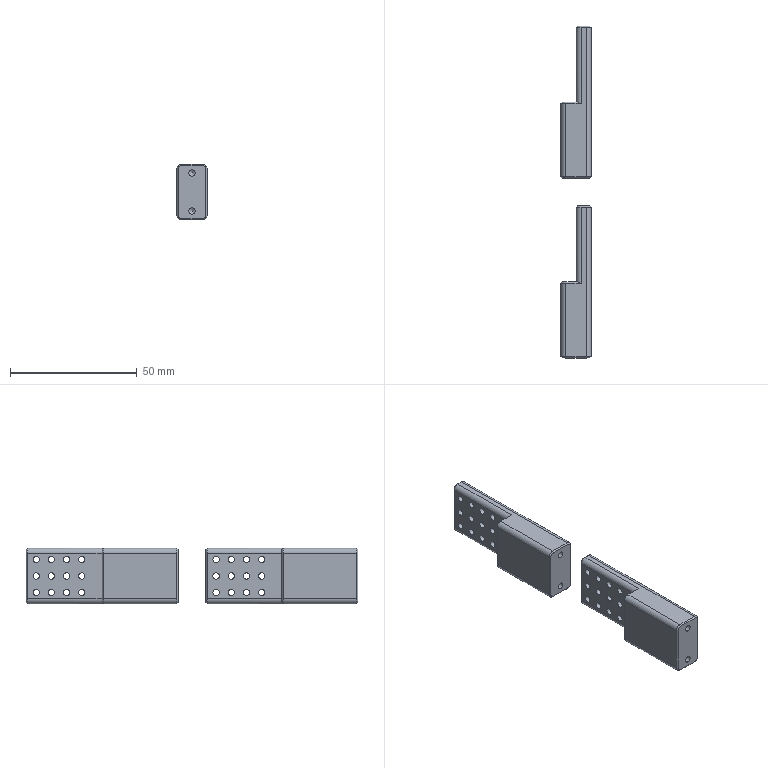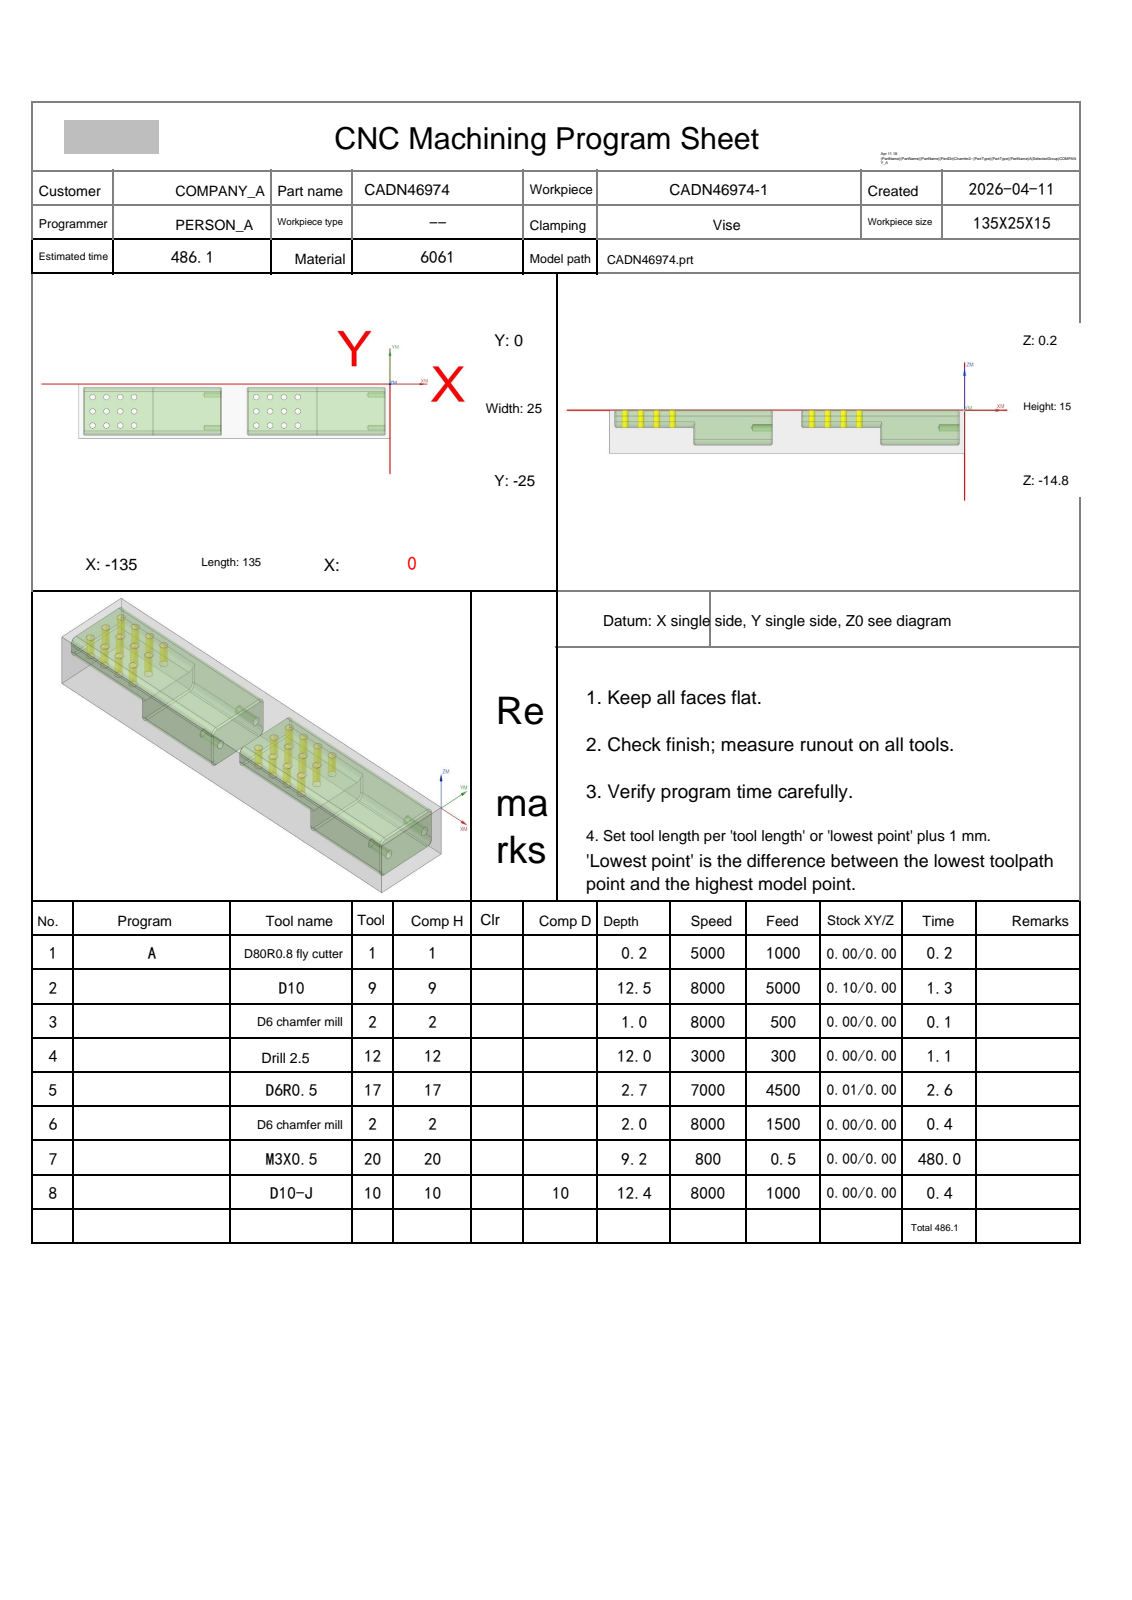NC program | NX | posted by the shop | part box 12 x 131 x 22 mm
Lines 673 to 2479 of 2479, first 1452 of 1807 lines:
N5 T17 M06
(D6R0.5  D=6. R=0.5 H=17 ce=0.01 di=0.00)
G00 G90 G54 X3.104 Y-17.401 M03 S7000
G43 H17 Z10.2
M08
Z.491
G01 Z-.009 F4500.
X3.1
G03 X.1 Y-20.397 I0.0 J-3.
G02 X.128 Y-20.959 I-5.567 J-.562
X.005 Y-22.127 I-5.596 J0.0
X-2.5 Y-24.221 I-2.59 J.553
G01 X-61.5
G02 X-64.069 Y-21.872 I.126 J2.717
G01 X-64.077 Y-21.814
X-64.091 Y-20.262
X-64.132 Z-.015
X-64.15 Z-.021
X-64.136 Y-21.732
G03 X-61.506 Y-24.336 I2.63 J.026
G01 X-2.5
G03 X.134 Y-21.627 I-.098 J2.73
G01 X.143 Y-20.397
X.193 Z-.038
X.185 Y-21.814
X.132 Y-22.159
G02 X-2.5 Y-24.443 I-2.718 J.473
G01 X-61.5
G02 X-64.184 Y-21.693 I.1 J2.782
G01 X-64.2 Y-20.262
X-64.224 Z-.048
X-64.242 Z-.058
X-64.227 Y-21.814
X-64.182 Y-22.159
G03 X-61.5 Y-24.546 I2.79 J.435
G01 X-2.5
G03 X.195 Y-22.071 I-.096 J2.81
G01 X.226 Y-21.814
X.24 Y-20.397
X.278 Z-.082
G02 X.304 Y-21.018 I-7.327 J-.621
X.184 Y-22.339 I-7.354 J0.0
X-2.5 Y-24.647 I-2.769 J.506
G01 X-61.5
G02 X-64.227 Y-22.159 I.094 J2.842
G01 X-64.269 Y-21.814
X-64.28 Y-20.298
X-64.317 Y-20.343 Z-.111
G03 X-64.341 Y-20.974 I8.456 J-.632
X-64.202 Y-22.504 I8.48 J0.0
X-61.5 Y-24.745 I2.81 J.639
G01 X-2.5
G03 X.219 Y-22.404 I-.075 J2.836
X.341 Y-21.019 I-7.816 J1.385
X.316 Y-20.397 I-7.937 J0.0
G01 X.342 Z-.127
X.359 Z-.143
X.349 Y-21.814
X.305 Y-22.159
G02 X-1.293 Y-24.55 I-3.063 J.317
X-2.5 Y-24.842 I-1.433 J3.287
G01 X-61.5
G02 X-64.034 Y-23.133 I.076 J2.846
G01 X-64.141 Y-22.84
G02 X-64.345 Y-21.713 I3.175 J1.158
G01 X-64.357 Y-20.394
X-64.395 Y-20.392 Z-.178
X-64.385 Y-21.656
G03 X-64.036 Y-23.254 I3.994 J.034
X-61.5 Y-24.937 I2.598 J1.163
G01 X-2.5
G03 X.065 Y-23.188 I-.07 J2.857
X.385 Y-21.633 I-3.774 J1.588
G01 X.395 Y-20.391
X.435 Z-.218
X.423 Y-21.814
X.384 Y-22.159
G02 X-.501 Y-24.157 I-3.438 J.329
X-2.478 Y-25.03 I-1.977 J1.801
G01 X-61.5
G02 X-63.948 Y-23.539 I.041 J2.822
X-64.387 Y-22.159 I3.309 J1.814
G01 X-64.422 Y-21.814
X-64.435 Y-20.394
X-64.478 Y-20.395 Z-.261
X-64.465 Y-21.814
G03 X-64.015 Y-23.539 I4.608 J.282
X-61.5 Y-25.122 I2.564 J1.285
G01 X-2.5
G03 X.009 Y-23.537 I-.042 J2.845
X.467 Y-21.615 I-3.965 J1.96
G01 X.478 Y-20.395
X.524 Y-20.397 Z-.307
X.513 Y-21.634
G02 X-.097 Y-23.837 I-4.424 J.04
X-2.499 Y-25.211 I-2.402 J1.412
G01 X-61.5
G02 X-64.066 Y-23.543 I.038 J2.866
X-64.514 Y-21.54 I4.451 J2.048
G01 X-64.524 Y-20.396
X-64.575 Y-20.398 Z-.357
G03 X-64.588 Y-20.988 I12.499 J-.59
X-64.562 Y-21.801 I12.513 J0.0
X-63.937 Y-23.884 I4.83 J.314
X-61.5 Y-25.298 I2.46 J1.433
G01 X-2.5
G03 X-.059 Y-23.884 I-.039 J2.882
X.567 Y-21.693 I-4.229 J2.392
X.582 Y-20.934 I-18.307 J.76
X.575 Y-20.398 I-18.323 J0.0
G01 X.628 Y-20.4 Z-.411
Y-21.469
G02 X-.004 Y-23.884 I-5.041 J.03
X-2.5 Y-25.383 I-2.519 J1.367
G01 X-61.5
G02 X-64.003 Y-23.879 I.031 J2.885
X-64.622 Y-21.633 I4.488 J2.447
X-64.636 Y-20.933 I17.84 J.7
X-64.628 Y-20.399 I17.853 J0.0
G01 X-64.685 Y-20.401 Z-.468
G03 X-64.693 Y-20.934 I17.258 J-.533
X-64.679 Y-21.641 I17.266 J0.0
X-63.845 Y-24.229 I5.08 J.208
X-61.5 Y-25.466 I2.373 J1.658
G01 X-2.5
G03 X-.063 Y-24.091 I-.032 J2.905
G01 X.054 Y-23.884
G03 X.667 Y-21.798 I-4.515 J2.46
X.698 Y-20.948 I-11.662 J.85
X.685 Y-20.401 I-11.693 J0.0
G01 X.745 Y-20.403 Z-.528
G02 X.758 Y-20.947 I-11.598 J-.544
X.694 Y-22.159 I-11.611 J0.0
X-.091 Y-24.229 I-5.507 J.906
X-2.5 Y-25.547 I-2.436 J1.593
G01 X-61.5
G02 X-63.901 Y-24.233 I.021 J2.89
X-64.729 Y-21.766 I4.355 J2.834
X-64.758 Y-20.947 I11.552 J.819
X-64.745 Y-20.399 I11.581 J0.0
G01 X-64.808 Y-20.406 Z-.591
G03 X-64.816 Y-20.874 I13.767 J-.467
X-64.756 Y-22.159 I13.775 J0.0
X-63.869 Y-24.368 I5.539 J.942
X-61.5 Y-25.625 I2.369 J1.604
G01 X-2.5
G03 X-.038 Y-24.229 I-.023 J2.91
X.757 Y-22.159 I-4.75 J3.012
X.821 Y-20.92 I-12.025 J1.239
X.808 Y-20.375 I-12.088 J0.0
G01 X.874 Y-20.415 Z-.658
G02 X.882 Y-20.873 I-13.64 J-.457
X.821 Y-22.159 I-13.648 J0.0
X.014 Y-24.229 I-5.474 J.943
G01 X-.22 Y-24.574
G02 X-2.5 Y-25.7 I-2.299 J1.786
G01 X-61.5
G02 X-63.687 Y-24.69 I.021 J2.917
X-64.82 Y-22.159 I4.359 J3.47
X-64.882 Y-20.878 I13.11 J1.282
X-64.874 Y-20.415 I13.173 J0.0
G01 X-64.909 Y-20.416 Z-.692
X-64.943 Y-20.417 Z-.727
G03 X-64.951 Y-20.882 I12.596 J-.464
X-64.886 Y-22.159 I12.605 J0.0
X-64.034 Y-24.288 I5.658 J1.031
G01 X-63.845 Y-24.574
G03 X-61.5 Y-25.772 I2.37 J1.744
G01 X-2.497
G03 X-.103 Y-24.488 I0.0 J2.872
G01 X.068 Y-24.229
G03 X.887 Y-22.159 I-4.524 J2.987
X.951 Y-20.876 I-12.929 J1.284
X.943 Y-20.417 I-12.992 J0.0
G01 X.979 Y-20.418 Z-.762
X1.013 Y-20.419 Z-.798
G02 X1.021 Y-20.863 I-12.618 J-.444
X.955 Y-22.159 I-12.626 J0.0
X.093 Y-24.276 I-5.299 J.922
X-2.5 Y-25.841 I-2.632 J1.43
G01 X-61.5
G02 X-63.9 Y-24.574 I.022 J2.948
G01 X-64.143 Y-24.196
G02 X-64.604 Y-23.345 I5.311 J3.423
X-65.011 Y-21.447 I4.296 J1.914
G01 X-65.013 Y-20.419
X-65.049 Y-20.42 Z-.833
X-65.084 Y-20.421 Z-.868
G03 X-65.092 Y-20.867 I11.906 J-.445
X-65.022 Y-22.159 I11.915 J0.0
X-64.034 Y-24.444 I5.388 J.974
X-61.5 Y-25.904 I2.56 J1.515
G01 X-2.5
G03 X-.323 Y-24.919 I-.013 J2.928
X.616 Y-23.44 I-5.066 J4.254
G01 X.662 Y-23.34
G03 X1.079 Y-21.464 I-4.106 J1.897
G01 X1.084 Y-20.422
X1.12 Y-20.423 Z-.904
X1.155 Y-20.424 Z-.939
G02 X1.162 Y-20.841 I-11.947 J-.417
X1.089 Y-22.159 I-11.954 J0.0
X-.001 Y-24.574 I-5.58 J1.065
X-2.5 Y-25.963 I-2.531 J1.611
G01 X-61.5
G02 X-64.034 Y-24.523 I.039 J3.017
X-65.09 Y-22.159 I4.492 J3.425
X-65.162 Y-20.837 I12.146 J1.322
X-65.155 Y-20.424 I12.217 J0.0
G01 X-65.191 Y-20.425 Z-.974
X-65.225 Y-20.426 Z-1.01
X-65.219 Y-21.469
G03 X-64.727 Y-23.47 I4.659 J.085
X-63.745 Y-24.966 I7.076 J3.575
X-61.503 Y-26.017 I2.242 J1.866
G01 X-2.5
G03 X-.215 Y-24.919 I-.02 J2.967
X.692 Y-23.539 I-6.554 J5.295
X1.219 Y-21.469 I-4.162 J2.162
G01 X1.226 Y-20.426
X1.261 Y-20.427 Z-1.045
X1.296 Y-20.428 Z-1.08
X1.289 Y-21.469
G02 X.753 Y-23.539 I-4.686 J.11
X-.262 Y-25.029 I-7.761 J4.197
X-2.497 Y-26.068 I-2.235 J1.884
G01 X-61.503
G02 X-63.757 Y-25.01 I0.0 J2.93
X-64.727 Y-23.588 I7.022 J5.833
X-65.288 Y-21.469 I4.103 J2.221
G01 X-65.296 Y-20.428
X-65.332 Y-20.429 Z-1.116
X-65.367 Y-20.43 Z-1.151
X-65.358 Y-21.469
G03 X-64.811 Y-23.539 I4.597 J.108
X-63.689 Y-25.132 I7.643 J4.191
X-61.504 Y-26.115 I2.185 J1.938
G01 X-2.5
G03 X-.253 Y-25.075 I-.024 J3.
G01 X-.128 Y-24.919
G03 X.787 Y-23.58 I-6.706 J5.558
X1.359 Y-21.469 I-4.009 J2.221
G01 X1.367 Y-20.43
X1.403 Y-20.431 Z-1.186
X1.438 Y-20.432 Z-1.222
X1.43 Y-21.431
G02 X.787 Y-23.671 I-4.346 J.036
X.184 Y-24.574 I-5.083 J2.737
X-.384 Y-25.264 I-6.247 J4.571
X-2.5 Y-26.159 I-2.14 J2.114
G01 X-61.5
G02 X-63.616 Y-25.264 I.024 J3.007
X-64.727 Y-23.782 I7.741 J6.956
X-65.427 Y-21.469 I3.958 J2.461
G01 X-65.431 Y-21.124
X-65.438 Y-20.432
X-65.473 Y-20.433 Z-1.257
X-65.508 Y-20.434 Z-1.293
X-65.497 Y-21.469
G03 X-64.924 Y-23.539 I4.366 J.095
X-63.687 Y-25.231 I9.099 J5.354
X-61.954 Y-26.162 I2.199 J2.016
G01 X-61.5 Y-26.199
X-2.5
X-2.272 Y-26.183
G03 X-.25 Y-25.158 I-.208 J2.918
G01 X-.048 Y-24.919
G03 X.924 Y-23.539 I-7.001 J5.959
X1.5 Y-21.469 I-3.831 J2.181
G01 X1.509 Y-20.434
X1.543 Y-20.583 Z-1.328
X1.576 Y-20.731 Z-1.363
X1.571 Y-21.469
G02 X.98 Y-23.539 I-4.32 J.114
X-.253 Y-25.202 I-9.003 J5.387
G01 X-.305 Y-25.264
G02 X-1.986 Y-26.19 I-2.21 J2.022
G01 X-2.5 Y-26.237
X-61.5
X-61.954 Y-26.201
G02 X-63.687 Y-25.274 I.469 J2.96
X-64.831 Y-23.791 I9.891 J8.817
X-65.547 Y-21.761 I3.655 J2.429
X-65.58 Y-21.027 I8.039 J.734
X-65.575 Y-20.727 I8.072 J0.0
G01 X-65.591 Y-20.896 Z-1.381
X-65.607 Y-21.064 Z-1.399
X-65.623 Y-21.232 Z-1.416
X-65.637 Y-21.401 Z-1.434
G03 X-65.037 Y-23.539 I4.149 J.01
X-63.653 Y-25.341 I9.631 J5.964
X-61.5 Y-26.271 I2.153 J2.028
G01 X-2.5
G03 X-.435 Y-25.431 I-.013 J2.991
X1.036 Y-23.539 I-8.047 J7.774
X1.641 Y-21.422 I-3.577 J2.168
G01 X1.649 Y-21.575 Z-1.444
X1.646 Y-21.729 Z-1.455
X1.639 Y-21.883 Z-1.465
X1.63 Y-22.037 Z-1.476
X1.615 Y-22.189 Z-1.486
X1.591 Y-22.339 Z-1.496
X1.559 Y-22.486 Z-1.507
G02 X.872 Y-23.884 I-4.54 J1.364
G01 X.44 Y-24.472
X.36 Y-24.574
X-.253 Y-25.281
G02 X-2.5 Y-26.304 I-2.264 J1.993
G01 X-61.503
G02 X-63.647 Y-25.381 I0.0 J2.95
X-64.874 Y-23.884 I9.924 J9.385
X-65.559 Y-22.49 I3.811 J2.74
G01 X-65.538 Y-22.628 Z-1.526
X-65.509 Y-22.765 Z-1.545
X-65.473 Y-22.898 Z-1.565
X-65.43 Y-23.028 Z-1.584
G03 X-64.927 Y-23.884 I4.787 J2.235
X-63.631 Y-25.43 I11.872 J8.636
X-61.502 Y-26.336 I2.13 J2.05
G01 X-2.5
G03 X-.401 Y-25.467 I-.006 J2.983
X.89 Y-23.93 I-10.286 J9.952
X1.431 Y-23.021 I-4.674 J3.398
G01 X1.402 Y-23.141 Z-1.611
X1.366 Y-23.257 Z-1.639
X1.317 Y-23.365 Z-1.666
G02 X.982 Y-23.884 I-3.452 J1.856
X-.382 Y-25.486 I-15.155 J11.531
X-2.5 Y-26.367 I-2.132 J2.139
G01 X-61.501
G02 X-63.631 Y-25.466 I0.0 J2.969
X-64.981 Y-23.884 I11.741 J11.393
X-65.32 Y-23.366 I3.833 J2.875
G01 X-65.281 Y-23.494 Z-1.709
X-65.228 Y-23.614 Z-1.752
G03 X-64.768 Y-24.229 I6.406 J4.313
G01 X-64.744 Y-24.252
G03 X-63.609 Y-25.518 I13.127 J10.626
X-61.503 Y-26.395 I2.106 J2.088
G01 X-2.5
G03 X-.593 Y-25.706 I-.016 J3.027
X-.392 Y-25.519 I-1.452 J1.765
G01 X-.149 Y-25.264
G03 X1.228 Y-23.618 I-10.789 J10.416
G01 X1.193 Y-23.718 Z-1.796
X1.148 Y-23.811 Z-1.84
G02 X-.253 Y-25.402 I-15.669 J12.394
G01 X-.289 Y-25.441
G02 X-2.495 Y-26.421 I-2.206 J1.993
G01 X-61.501
G02 X-63.626 Y-25.53 I0.0 J2.98
X-65.074 Y-23.911 I16.403 J16.117
G01 X-65.151 Y-23.805
X-65.12 Y-23.891 Z-1.886
X-65.081 Y-23.969 Z-1.931
G03 X-63.645 Y-25.538 I27.351 J23.594
X-61.502 Y-26.444 I2.144 J2.081
G01 X-2.496
G03 X-.28 Y-25.459 I0.0 J2.984
G01 X-.253 Y-25.429
G03 X1.098 Y-23.944 I-19.21 J18.822
G01 X1.058 Y-24.044 Z-2.026
G02 X-.332 Y-25.538 I-29.21 J25.791
X-2.5 Y-26.465 I-2.171 J2.08
G01 X-61.5
G02 X-63.687 Y-25.518 I.005 J3.012
X-65.043 Y-24.066 I34.442 J33.526
G01 X-65.005 Y-24.154 Z-2.122
G03 X-63.616 Y-25.609 I50.137 J46.44
X-61.5 Y-26.481 I2.122 J2.146
G01 X-2.5
G03 X-.383 Y-25.609 I-.006 J3.019
X1.012 Y-24.141 I-43.047 J42.298
G01 X.963 Y-24.23 Z-2.217
G03 X.44 Y-24.774 I18.578 J-18.365
G01 X.305 Y-24.919
G02 X-.446 Y-25.678 I-34.783 J33.665
X-2.5 Y-26.494 I-2.057 J2.184
G01 X-61.5
G02 X-63.629 Y-25.609 I.013 J3.035
X-64.963 Y-24.232 I99.236 J97.412
G01 X-64.939 Y-24.279 Z-2.311
X-64.858 Y-24.364
X-63.636 Y-25.609
G03 X-61.5 Y-26.503 I2.157 J2.156
G01 X-2.5
G03 X-.36 Y-25.609 I-.018 J3.051
G01 X-.315 Y-25.556
X-.253 Y-25.494
X.938 Y-24.278
X.926 Y-24.307 Z-2.406
X-.362 Y-25.614
G02 X-2.5 Y-26.508 I-2.138 J2.108
G01 X-61.506
G02 X-63.632 Y-25.619 I0.0 J2.987
G01 X-64.925 Y-24.309
X-64.915 Y-24.335 Z-2.5
X-64.677 Y-24.574
X-63.586 Y-25.67
G03 X-61.5 Y-26.51 I2.088 J2.174
G01 X-2.5
G03 X-.423 Y-25.678 I0.0 J3.007
G01 X.915 Y-24.333
G00 Z10.2
X-67.104 Y-7.564
Z.491
G01 Z-.009
X-67.094
G03 X-64.094 Y-4.601 I0.0 J3.
G01 X-64.077 Y-3.186
X-64.063 Y-3.091
G02 X-61.5 Y-.779 I2.687 J-.403
G01 X-2.5
G02 X.081 Y-3.186 I-.124 J-2.72
G01 X.093 Y-3.316
X.101 Y-4.6
X.148 Z-.021
X.134 Y-3.365
G03 X-2.5 Y-.664 I-2.733 J-.031
G01 X-61.507
G03 X-64.136 Y-3.268 I0.0 J-2.629
G01 X-64.149 Y-4.599
X-64.199 Z-.038
X-64.182 Y-3.186
X-64.149 Y-2.943
G02 X-61.5 Y-.557 I2.739 J-.377
G01 X-2.5
G02 X.132 Y-2.841 I-.085 J-2.757
G01 X.185 Y-3.186
X.197 Y-4.6
X.241 Z-.058
X.226 Y-3.186
X.195 Y-2.929
G03 X-2.5 Y-.454 I-2.791 J-.335
G01 X-61.5
G03 X-64.182 Y-2.841 I.108 J-2.822
G01 X-64.227 Y-3.186
X-64.24 Y-4.599
X-64.266 Y-4.6 Z-.07
X-64.282 Y-4.601 Z-.082
X-64.269 Y-3.186
X-64.227 Y-2.841
G02 X-61.5 Y-.353 I2.821 J-.354
G01 X-2.5
G02 X.226 Y-2.841 I-.105 J-2.853
G01 X.272 Y-3.186
X.283 Y-4.6
X.32 Z-.111
X.312 Y-3.186
X.272 Y-2.841
G03 X-2.5 Y-.255 I-2.874 J-.302
G01 X-61.5
G03 X-64.202 Y-2.496 I.108 J-2.88
X-64.34 Y-4.003 I8.134 J-1.507
X-64.319 Y-4.601 I8.272 J0.0
G01 X-64.342 Y-4.6 Z-.127
X-64.357 Y-4.599 Z-.143
X-64.344 Y-3.186
X-64.31 Y-2.841
G02 X-62.647 Y-.418 I3.103 J-.348
X-61.5 Y-.158 I1.423 J-3.623
G01 X-2.5
G02 X-.003 Y-1.801 I-.058 J-2.807
X.351 Y-3.404 I-3.58 J-1.63
G01 X.359 Y-4.6
X.395 Y-4.631 Z-.178
G03 X.414 Y-4.04 I-9.48 J.591
X.287 Y-2.496 I-9.498 J0.0
X-2.5 Y-.063 I-2.904 J-.515
G01 X-61.5
G03 X-63.324 Y-.771 I.083 J-2.92
X-64.347 Y-2.841 I2.273 J-2.41
G01 X-64.383 Y-3.186
X-64.395 Y-4.608
X-64.435 Y-4.606 Z-.218
X-64.422 Y-3.186
X-64.387 Y-2.841
G02 X-63.493 Y-.84 I3.472 J-.351
X-61.522 Y.03 I1.971 J-1.798
G01 X-2.5
G02 X.095 Y-1.75 I-.057 J-2.864
X.424 Y-3.392 I-4.11 J-1.68
G01 X.435 Y-4.604
X.478 Y-4.606 Z-.261
X.467 Y-3.385
G03 X.009 Y-1.463 I-4.423 J-.038
X-2.5 Y.122 I-2.551 J-1.261
G01 X-61.5
G03 X-64.015 Y-1.461 I.049 J-2.868
X-64.465 Y-3.186 I4.158 J-2.007
G01 X-64.478 Y-4.605
X-64.501 Y-4.604 Z-.284
X-64.524 Z-.307
X-64.514 Y-3.46
G02 X-64.066 Y-1.457 I4.9 J-.045
X-61.5 Y.211 I2.604 J-1.198
G01 X-2.5
G02 X-.085 Y-1.184 I0.0 J-2.788
X.512 Y-3.186 I-3.911 J-2.256
G01 X.524 Y-4.605
X.575 Y-4.603 Z-.357
G03 X.582 Y-4.069 I-18.545 J.534
X.567 Y-3.309 I-18.553 J0.0
X-.059 Y-1.116 I-4.854 J-.199
X-2.5 Y.298 I-2.48 J-1.468
G01 X-61.5
G03 X-63.937 Y-1.116 I.024 J-2.847
X-64.561 Y-3.186 I4.205 J-2.398
X-64.582 Y-4.067 I18.267 J-.881
X-64.575 Y-4.602 I18.288 J0.0
G01 X-64.601 Z-.384
X-64.628 Y-4.601 Z-.411
G02 X-64.636 Y-4.066 I17.668 J.535
X-64.622 Y-3.365 I17.676 J0.0
X-64.003 Y-1.121 I5.109 J-.203
X-61.5 Y.383 I2.534 J-1.381
G01 X-2.5
G02 X-.004 Y-1.116 I-.023 J-2.866
X.628 Y-3.531 I-4.409 J-2.445
G01 Y-4.602
X.685 Y-4.6 Z-.468
G03 X.698 Y-4.05 I-11.6 J.55
X.667 Y-3.195 I-11.613 J0.0
X.021 Y-1.058 I-5.111 J-.377
G01 X-.063 Y-.909
G03 X-2.5 Y.466 I-2.47 J-1.53
G01 X-61.5
G03 X-63.845 Y-.771 I.028 J-2.895
X-64.679 Y-3.357 I4.247 J-2.797
X-64.693 Y-4.065 I17.096 J-.708
X-64.685 Y-4.599 I17.111 J0.0
G01 X-64.745 Y-4.601 Z-.528
G02 X-64.758 Y-4.058 I11.732 J.544
X-64.729 Y-3.236 I11.745 J0.0
X-63.901 Y-.767 I5.18 J-.363
X-61.5 Y.547 I2.422 J-1.577
G01 X-2.5
G02 X-.091 Y-.771 I-.027 J-2.911
X.694 Y-2.841 I-4.722 J-2.976
X.758 Y-4.05 I-11.438 J-1.21
X.745 Y-4.598 I-11.502 J0.0
G01 X.808 Y-4.626 Z-.591
G03 X.821 Y-4.071 I-11.761 J.555
X.757 Y-2.841 I-11.774 J0.0
X-.038 Y-.771 I-5.545 J-.942
X-2.5 Y.625 I-2.485 J-1.515
G01 X-61.5
G03 X-63.869 Y-.632 I0.0 J-2.861
X-64.756 Y-2.841 I4.653 J-3.152
X-64.816 Y-4.128 I13.787 J-1.288
X-64.808 Y-4.594 I13.847 J0.0
G01 X-64.842 Y-4.589 Z-.624
X-64.874 Y-4.585 Z-.658
G02 X-64.882 Y-4.129 I13.336 J.456
X-64.82 Y-2.841 I13.343 J0.0
X-63.687 Y-.31 I5.493 J-.941
X-61.5 Y.7 I2.208 J-1.907
G01 X-2.5
G02 X-.22 Y-.426 I-.019 J-2.911
G01 X-.049 Y-.678
G02 X.821 Y-2.841 I-4.572 J-3.096
X.882 Y-4.124 I-13.479 J-1.283
X.874 Y-4.586 I-13.54 J0.0
G01 X.909 Y-4.585 Z-.692
X.942 Y-4.584 Z-.727
X.943 Y-3.876
X.941 Y-3.531
G03 X.093 Y-.81 I-5.137 J-.108
G01 X.068 Y-.771
G03 X-2.5 Y.772 I-2.6 J-1.419
G01 X-61.507
G03 X-63.909 Y-.522 I0.0 J-2.876
G01 X-64.034 Y-.712
G03 X-64.886 Y-2.841 I4.809 J-3.162
X-64.951 Y-4.128 I12.765 J-1.287
X-64.943 Y-4.583 I12.83 J0.0
G01 X-64.979 Y-4.582 Z-.762
X-65.014 Y-4.581 Z-.798
X-65.011 Y-3.531
G02 X-64.51 Y-1.461 I4.683 J-.038
X-64.034 Y-.634 I4.75 J-2.182
X-61.5 Y.841 I2.559 J-1.483
G01 X-2.5
G02 X.093 Y-.724 I-.038 J-2.995
X.954 Y-2.841 I-4.435 J-3.037
X1.021 Y-4.136 I-12.618 J-1.296
X1.013 Y-4.581 I-12.684 J0.0
G01 X1.049 Y-4.58 Z-.833
X1.084 Y-4.579 Z-.868
X1.079 Y-3.506
G03 X.723 Y-1.793 I-4.381 J-.017
X-.205 Y-.219 I-6.635 J-2.852
X-2.497 Y.904 I-2.292 J-1.778
G01 X-61.5
G03 X-64.034 Y-.556 I.026 J-2.974
X-65.022 Y-2.841 I4.405 J-3.262
X-65.092 Y-4.146 I12.137 J-1.305
X-65.085 Y-4.578 I12.207 J0.0
G01 X-65.121 Y-4.577 Z-.904
X-65.155 Y-4.576 Z-.939
G02 X-65.163 Y-4.155 I11.947 J.421
X-65.09 Y-2.841 I11.955 J0.0
X-64.034 Y-.477 I5.555 J-1.066
X-61.5 Y.963 I2.573 J-1.577
G01 X-2.5
G02 X-.001 Y-.426 I-.031 J-3.
X1.089 Y-2.841 I-4.49 J-3.479
X1.162 Y-4.145 I-11.551 J-1.304
X1.154 Y-4.577 I-11.624 J0.0
G01 X1.19 Y-4.575 Z-.974
X1.225 Y-4.574 Z-1.01
X1.218 Y-3.531
G03 X.692 Y-1.461 I-4.689 J-.091
X-.215 Y-.081 I-7.45 J-3.908
X-2.5 Y1.017 I-2.304 J-1.868
G01 X-61.503
G03 X-63.745 Y-.034 I0.0 J-2.917
X-64.727 Y-1.53 I6.094 J-5.072
X-65.22 Y-3.531 I4.172 J-2.089
G01 X-65.226 Y-4.574
X-65.262 Y-4.573 Z-1.045
X-65.297 Y-4.572 Z-1.08
X-65.29 Y-3.531
G02 X-64.727 Y-1.412 I4.676 J-.108
X-63.758 Y.008 I7.994 J-4.412
X-61.502 Y1.068 I2.256 J-1.873
G01 X-2.497
G02 X-.263 Y.029 I0.0 J-2.923
X.752 Y-1.461 I-6.732 J-5.678
X1.288 Y-3.531 I-4.143 J-2.176
G01 X1.296 Y-4.572
X1.331 Y-4.571 Z-1.116
X1.366 Y-4.57 Z-1.151
X1.358 Y-3.531
G03 X.787 Y-1.421 I-4.567 J-.104
X-.128 Y-.081 I-7.609 J-4.21
G01 X-.253 Y.075
G03 X-2.5 Y1.115 I-2.271 J-1.96
G01 X-61.503
G03 X-63.689 Y.132 I0.0 J-2.921
X-64.811 Y-1.461 I6.523 J-5.784
X-65.36 Y-3.531 I4.068 J-2.187
G01 X-65.368 Y-4.57
X-65.403 Y-4.569 Z-1.186
X-65.439 Y-4.568 Z-1.222
X-65.435 Y-3.876
X-65.43 Y-3.531
G02 X-64.727 Y-1.218 I4.68 J-.16
X-63.616 Y.264 I8.855 J-5.475
X-61.5 Y1.159 I2.141 J-2.114
G01 X-2.5
G02 X-.253 Y.12 I-.022 J-2.998
X.295 Y-.568 I-12.955 J-10.877
X1.029 Y-1.792 I-5.36 J-4.044
X1.427 Y-3.531 I-3.916 J-1.812
G01 X1.437 Y-4.567
X1.507 Y-4.532 Z-1.293
X1.497 Y-3.531
G03 X.923 Y-1.461 I-4.374 J-.097
X-.048 Y-.081 I-7.945 J-4.558
G01 X-.251 Y.159
G03 X-2.27 Y1.183 I-2.226 J-1.889
G01 X-2.5 Y1.199
X-61.5
X-61.954 Y1.162
G03 X-63.687 Y.231 I.468 J-2.951
X-64.924 Y-1.461 I7.866 J-7.049
X-65.501 Y-3.531 I3.83 J-2.182
G01 X-65.509 Y-4.566
X-65.544 Y-4.416 Z-1.328
X-65.577 Y-4.267 Z-1.363
X-65.572 Y-3.531
G02 X-64.981 Y-1.461 I4.303 J-.109
X-63.696 Y.264 I9.768 J-5.937
X-61.954 Y1.201 I2.209 J-2.02
G01 X-61.5 Y1.237
X-2.5
G02 X-1.324 Y.989 I-.05 J-3.154
X-.344 Y.301 I-1.103 J-2.616
X.899 Y-1.322 I-8.053 J-7.452
X1.546 Y-3.24 I-3.691 J-2.314
X1.58 Y-3.969 I-7.987 J-.729
X1.574 Y-4.263 I-8.021 J0.0
G01 X1.591 Y-4.098 Z-1.381
X1.606 Y-3.933 Z-1.399
X1.622 Y-3.768 Z-1.416
X1.637 Y-3.604 Z-1.434
G03 X1.036 Y-1.461 I-4.125 J-.001
X-.43 Y.427 I-9.571 J-5.917
X-2.5 Y1.271 I-2.083 J-2.149
G01 X-61.501
G03 X-63.652 Y.342 I0.0 J-2.956
X-65.037 Y-1.461 I8.234 J-7.759
X-65.643 Y-3.569 I3.612 J-2.178
G01 X-65.649 Y-3.417 Z-1.444
X-65.646 Y-3.264 Z-1.455
X-65.639 Y-3.111 Z-1.465
X-65.63 Y-2.957 Z-1.476
X-65.614 Y-2.805 Z-1.486
X-65.59 Y-2.656 Z-1.496
X-65.559 Y-2.509 Z-1.507
G02 X-64.874 Y-1.116 I4.502 J-1.35
X-63.649 Y.379 I11.156 J-7.892
X-61.501 Y1.304 I2.147 J-2.03
G01 X-2.5
G02 X-.414 Y.444 I-.008 J-2.979
X.872 Y-1.116 I-9.23 J-8.92
X1.559 Y-2.515 I-3.83 J-2.748
G01 X1.539 Y-2.377 Z-1.526
X1.51 Y-2.242 Z-1.545
X1.475 Y-2.109 Z-1.565
X1.431 Y-1.981 Z-1.584
G03 X.885 Y-1.062 I-5.197 J-2.471
X-.397 Y.462 I-11.618 J-8.465
X-2.5 Y1.336 I-2.109 J-2.108
G01 X-61.501
G03 X-63.632 Y.429 I0.0 J-2.957
X-64.927 Y-1.116 I10.584 J-10.186
X-65.43 Y-1.972 I4.283 J-3.091
G01 X-65.401 Y-1.855 Z-1.611
X-65.366 Y-1.741 Z-1.639
X-65.32 Y-1.634 Z-1.666
G02 X-64.981 Y-1.116 I4.174 J-2.358
X-63.63 Y.467 I13.102 J-9.821
X-61.502 Y1.367 I2.128 J-2.065
G01 X-2.496
G02 X-.354 Y.452 I0.0 J-2.965
X.983 Y-1.116 I-12.954 J-12.397
X1.319 Y-1.639 I-3.203 J-2.425
G01 X1.281 Y-1.509 Z-1.709
X1.23 Y-1.386 Z-1.752
G03 X.787 Y-.799 I-5.878 J-3.977
X-.364 Y.496 I-18.691 J-15.453
X-2.5 Y1.395 I-2.149 J-2.118
G01 X-61.5
G03 X-63.687 Y.442 I.013 J-3.016
X-64.473 Y-.426 I11.794 J-11.47
G01 X-64.744 Y-.748
G03 X-65.228 Y-1.386 I4.764 J-4.12
G01 X-65.197 Y-1.285 Z-1.796
X-65.151 Y-1.195 Z-1.84
X-65.096 Y-1.116
X-64.805 Y-.762
X-64.768 Y-.724
G02 X-63.622 Y.534 I16.31 J-13.693
X-61.502 Y1.421 I2.121 J-2.091
G01 X-2.5
G02 X-.283 Y.435 I0.0 J-2.984
G01 X-.253 Y.402
X-.067 Y.208
G02 X1.15 Y-1.191 I-13.413 J-12.897
G01 X1.078 Y-1.058 Z-1.886
X.994 Y-.934 Z-1.931
G03 X-.253 Y.429 I-20.525 J-17.526
G01 X-.338 Y.524
G03 X-2.5 Y1.444 I-2.171 J-2.1
G01 X-61.502
G03 X-63.645 Y.539 I0.0 J-2.986
X-65.081 Y-1.031 I25.879 J-25.129
G01 X-65.036 Y-.949 Z-1.979
X-64.987 Y-.87 Z-2.026
G02 X-63.687 Y.518 I39.056 J-35.279
X-61.5 Y1.465 I2.191 J-2.062
G01 X-2.5
G02 X-.328 Y.534 I-.004 J-3.007
X1.017 Y-.907 I-29.925 J-29.284
G01 X1.028 Y-.892 Z-2.074
X1.034 Y-.884 Z-2.122
G03 X-.384 Y.609 I-41.583 J-38.072
X-2.5 Y1.481 I-2.119 J-2.139
G01 X-61.5
G03 X-63.616 Y.609 I.006 J-3.019
X-65.004 Y-.845 I48.618 J-47.761
G01 X-64.963 Y-.769 Z-2.217
X-64.883 Y-.685
X-63.687 Y.55
X-63.629 Y.609
G02 X-61.5 Y1.494 I2.142 J-2.149
G01 X-2.5
G02 X-.373 Y.609 I-.004 J-3.008
X.932 Y-.74 I-71.305 J-70.306
G01 X.962 Y-.768
X.938 Y-.722 Z-2.311
G03 X-.419 Y.663 I-187.5 J-182.469
X-2.5 Y1.503 I-2.095 J-2.192
G01 X-61.5
G03 X-63.636 Y.609 I.021 J-3.049
G01 X-64.939 Y-.722
X-64.925 Y-.692 Z-2.406
X-63.629 Y.62
G02 X-61.501 Y1.508 I2.127 J-2.102
G01 X-2.497
G02 X-.363 Y.615 I0.0 J-2.996
G01 X.926 Y-.693
X.915 Y-.667 Z-2.5
X-.352 Y.609
G03 X-2.5 Y1.51 I-2.149 J-2.112
G01 X-61.5
G03 X-63.647 Y.609 I.001 J-3.01
G01 X-64.872 Y-.622
X-64.915 Y-.666
G00 Z10.2
X-67.896 Y-17.436
Z.491
G01 Z-.009
X-67.906
G03 X-70.906 Y-20.399 I0.0 J-3.
G01 X-70.923 Y-21.814
X-70.937 Y-21.909
G02 X-73.5 Y-24.221 I-2.687 J.403
G01 X-132.5
G02 X-135.08 Y-21.814 I.124 J2.719
G01 X-135.093 Y-21.684
X-135.101 Y-20.4
X-135.148 Z-.021
X-135.134 Y-21.635
G03 X-132.5 Y-24.336 I2.733 J.031
G01 X-73.493
G03 X-70.864 Y-21.732 I0.0 J2.629
G01 X-70.851 Y-20.401
X-70.801 Z-.038
X-70.818 Y-21.814
X-70.851 Y-22.057
G02 X-73.5 Y-24.443 I-2.739 J.377
G01 X-132.5
G02 X-135.132 Y-22.159 I.085 J2.757
G01 X-135.185 Y-21.814
X-135.197 Y-20.4
X-135.223 Z-.048
X-135.241 Z-.058
X-135.226 Y-21.814
X-135.195 Y-22.071
G03 X-132.5 Y-24.546 I2.791 J.335
G01 X-73.5
G03 X-70.818 Y-22.159 I-.108 J2.822
G01 X-70.773 Y-21.814
X-70.76 Y-20.401
X-70.734 Y-20.4 Z-.07
X-70.718 Y-20.399 Z-.082
X-70.731 Y-21.814
X-70.773 Y-22.159
G02 X-73.5 Y-24.647 I-2.821 J.354
G01 X-132.5
G02 X-135.226 Y-22.159 I.105 J2.853
G01 X-135.272 Y-21.814
X-135.283 Y-20.4
X-135.305 Z-.096
X-135.32 Z-.111
X-135.312 Y-21.814
X-135.272 Y-22.159
G03 X-132.5 Y-24.745 I2.874 J.302
G01 X-73.5
G03 X-70.798 Y-22.504 I-.108 J2.88
X-70.66 Y-20.997 I-8.131 J1.507
X-70.681 Y-20.399 I-8.27 J0.0
G01 X-70.658 Y-20.4 Z-.127
X-70.643 Y-20.401 Z-.143
X-70.655 Y-21.814
X-70.69 Y-22.159
G02 X-72.353 Y-24.582 I-3.103 J.348
X-73.5 Y-24.842 I-1.423 J3.623
G01 X-132.5
G02 X-134.997 Y-23.199 I.058 J2.807
X-135.351 Y-21.596 I3.58 J1.63
G01 X-135.359 Y-20.4
X-135.395 Y-20.37 Z-.178
G03 X-135.414 Y-20.96 I9.474 J-.591
X-135.287 Y-22.504 I9.493 J0.0
X-132.5 Y-24.937 I2.904 J.515
G01 X-73.5
G03 X-71.676 Y-24.229 I-.083 J2.92
X-70.653 Y-22.159 I-2.273 J2.41
G01 X-70.616 Y-21.814
X-70.605 Y-20.392
X-70.565 Y-20.394 Z-.218
X-70.577 Y-21.814
X-70.613 Y-22.159
G02 X-71.507 Y-24.16 I-3.472 J.351
X-73.478 Y-25.03 I-1.971 J1.798
G01 X-132.5
G02 X-135.095 Y-23.25 I.057 J2.864
X-135.424 Y-21.608 I4.11 J1.68
G01 X-135.435 Y-20.397
X-135.478 Y-20.395 Z-.261
X-135.467 Y-21.617
G03 X-135.01 Y-23.537 I4.414 J.038
X-132.5 Y-25.122 I2.553 J1.263
G01 X-73.5
G03 X-70.985 Y-23.539 I-.049 J2.868
X-70.535 Y-21.814 I-4.166 J2.01
G01 X-70.522 Y-20.395
X-70.476 Y-20.396 Z-.307
X-70.486 Y-21.537
G02 X-70.934 Y-23.542 I-4.906 J.044
X-73.5 Y-25.211 I-2.605 J1.197
G01 X-132.503
G02 X-134.912 Y-23.822 I0.0 J2.783
X-135.512 Y-21.814 I3.908 J2.262
G01 X-135.524 Y-20.396
X-135.575 Y-20.398 Z-.357
G03 X-135.582 Y-20.932 I18.514 J-.534
X-135.567 Y-21.692 I18.522 J0.0
X-134.941 Y-23.884 I4.854 J.199
X-132.5 Y-25.298 I2.48 J1.468
G01 X-73.5
G03 X-71.063 Y-23.884 I-.023 J2.847
X-70.439 Y-21.814 I-4.211 J2.4
X-70.418 Y-20.934 I-18.448 J.881
X-70.425 Y-20.398 I-18.469 J0.0
G01 X-70.372 Y-20.399 Z-.411
G02 X-70.364 Y-20.934 I-17.812 J-.535
X-70.377 Y-21.631 I-17.82 J0.0
X-70.997 Y-23.879 I-5.114 J.2
X-73.5 Y-25.383 I-2.533 J1.38
G01 X-132.5
G02 X-134.996 Y-23.884 I.024 J2.867
X-135.628 Y-21.469 I4.409 J2.445
G01 Y-20.399
X-135.685 Y-20.401 Z-.468
Y-21.469
G03 X-134.747 Y-24.36 I5.041 J.038
X-132.5 Y-25.466 I2.275 J1.787
G01 X-73.5
G03 X-71.155 Y-24.229 I-.028 J2.895
X-70.321 Y-21.641 I-4.247 J2.797
X-70.307 Y-20.935 I-17.163 J.706
X-70.315 Y-20.401 I-17.178 J0.0
G01 X-70.255 Y-20.399 Z-.528
G02 X-70.242 Y-20.942 I-11.736 J-.544
X-70.271 Y-21.764 I-11.749 J0.0
X-71.099 Y-24.234 I-5.179 J.363
X-73.5 Y-25.547 I-2.422 J1.577
G01 X-132.5
G02 X-134.909 Y-24.229 I.027 J2.911
X-135.694 Y-22.159 I4.722 J2.976
X-135.758 Y-20.95 I11.428 J1.209
X-135.745 Y-20.403 I11.491 J0.0
G01 X-135.808 Y-20.375 Z-.591
G03 X-135.821 Y-20.93 I11.745 J-.554
X-135.757 Y-22.159 I11.758 J0.0
X-134.962 Y-24.229 I5.547 J.943
X-132.5 Y-25.625 I2.485 J1.515
G01 X-73.498
G03 X-71.133 Y-24.371 I0.0 J2.858
X-70.244 Y-22.159 I-4.651 J3.154
X-70.184 Y-20.87 I-13.826 J1.289
X-70.192 Y-20.406 I-13.886 J0.0
G01 X-70.158 Y-20.411 Z-.624
X-70.126 Y-20.415 Z-.658
G02 X-70.118 Y-20.872 I-13.347 J-.457
X-70.18 Y-22.159 I-13.355 J0.0
X-71.287 Y-24.659 I-5.513 J.946
X-73.5 Y-25.7 I-2.233 J1.876
G01 X-132.5
G02 X-134.78 Y-24.574 I.019 J2.911
G01 X-134.951 Y-24.322
G02 X-135.821 Y-22.159 I4.572 J3.096
X-135.882 Y-20.877 I13.443 J1.282
X-135.874 Y-20.415 I13.504 J0.0
G01 X-135.909 Y-20.416 Z-.692
X-135.943 Y-20.417 Z-.727
G03 X-135.951 Y-20.883 I12.777 J-.466
X-135.887 Y-22.159 I12.786 J0.0
X-135.068 Y-24.229 I5.343 J.917
G01 X-134.839 Y-24.574
G03 X-132.5 Y-25.772 I2.357 J1.718
G01 X-73.5
G03 X-71.185 Y-24.61 I0.0 J2.886
X-70.62 Y-23.673 I-4.521 J3.366
X-70.059 Y-21.469 I-4.179 J2.236
G01 X-70.057 Y-20.417
X-70.021 Y-20.418 Z-.762
X-69.987 Y-20.419 Z-.798
X-69.99 Y-21.467
G02 X-70.391 Y-23.33 I-4.595 J.014
X-71.162 Y-24.657 I-6.635 J2.97
X-73.497 Y-25.841 I-2.335 J1.711
G01 X-132.5
G02 X-135.093 Y-24.276 I.038 J2.995
X-135.955 Y-22.159 I4.435 J3.038
X-136.022 Y-20.873 I12.284 J1.286
X-136.013 Y-20.419 I12.351 J0.0
G01 X-136.049 Y-20.42 Z-.833
X-136.084 Y-20.422 Z-.868
X-136.08 Y-21.494
G03 X-135.723 Y-23.207 I4.38 J.017
X-134.795 Y-24.781 I6.639 J2.855
X-132.503 Y-25.904 I2.292 J1.777
G01 X-73.5
G03 X-71.05 Y-24.574 I-.023 J2.965
G01 X-71.01 Y-24.514
G03 X-69.978 Y-22.159 I-4.554 J3.4
X-69.908 Y-20.855 I-12.154 J1.304
X-69.916 Y-20.421 I-12.223 J0.0
G01 X-69.88 Y-20.423 Z-.904
X-69.845 Y-20.424 Z-.939
X-69.85 Y-21.469
G02 X-70.367 Y-23.539 I-4.73 J.082
X-71.214 Y-24.86 I-6.977 J3.544
X-73.498 Y-25.963 I-2.283 J1.812
G01 X-132.5
G02 X-134.999 Y-24.574 I.031 J3.
X-136.089 Y-22.159 I4.485 J3.477
X-136.163 Y-20.853 I11.565 J1.306
X-136.155 Y-20.424 I11.639 J0.0
G01 X-136.191 Y-20.425 Z-.974
X-136.225 Y-20.426 Z-1.01
X-136.219 Y-21.469
G03 X-135.692 Y-23.539 I4.684 J.09
X-134.785 Y-24.919 I7.469 J3.921
X-132.5 Y-26.017 I2.305 J1.869
G01 X-73.494
G03 X-71.161 Y-24.851 I0.0 J2.918
G01 X-71.119 Y-24.796
G03 X-70.273 Y-23.47 I-6.124 J4.84
X-69.781 Y-21.469 I-4.175 J2.089
G01 X-69.774 Y-20.426
X-69.739 Y-20.427 Z-1.045
X-69.704 Y-20.428 Z-1.08
X-69.711 Y-21.469
G02 X-70.273 Y-23.588 I-4.678 J.107
X-71.094 Y-24.816 I-6.927 J3.746
G01 X-71.109 Y-24.836
G02 X-73.499 Y-26.068 I-2.39 J1.703
G01 X-132.502
G02 X-134.739 Y-25.028 I0.0 J2.925
X-135.753 Y-23.539 I6.753 J5.691
X-136.288 Y-21.469 I4.138 J2.175
G01 X-136.296 Y-20.428
X-136.332 Y-20.429 Z-1.116
X-136.367 Y-20.43 Z-1.151
X-136.358 Y-21.469
G03 X-135.787 Y-23.58 I4.559 J.102
X-134.872 Y-24.919 I7.627 J4.224
G01 X-134.747 Y-25.075
G03 X-132.5 Y-26.115 I2.273 J1.965
G01 X-73.5
G03 X-71.069 Y-24.836 I-.022 J2.99
X-70.027 Y-23.194 I-5.236 J4.479
X-69.641 Y-21.469 I-4.014 J1.803
G01 X-69.633 Y-20.43
X-69.597 Y-20.431 Z-1.186
X-69.562 Y-20.432 Z-1.222
X-69.571 Y-21.469
G02 X-69.966 Y-23.194 I-4.276 J.072
X-71.045 Y-24.856 I-6.61 J3.11
X-73.5 Y-26.159 I-2.482 J1.713
G01 X-132.5
G02 X-134.747 Y-25.12 I.022 J2.998
X-135.3 Y-24.425 I12.972 J10.891
X-136.029 Y-23.207 I5.343 J4.028
X-136.428 Y-21.469 I3.914 J1.811
G01 X-136.438 Y-20.432
X-136.473 Y-20.433 Z-1.257
X-136.508 Y-20.434 Z-1.293
X-136.497 Y-21.469
G03 X-135.924 Y-23.539 I4.368 J.095
X-134.953 Y-24.919 I7.98 J4.586
G01 X-134.749 Y-25.159
G03 X-132.73 Y-26.183 I2.226 J1.889
G01 X-132.5 Y-26.199
X-73.5
G03 X-72.353 Y-25.966 I-.066 J3.265
X-71.313 Y-25.231 I-1.209 J2.815
G01 X-71.05 Y-24.919
G03 X-70.205 Y-23.763 I-8.724 J7.256
X-69.499 Y-21.379 I-3.8 J2.422
G01 X-69.491 Y-20.434
X-69.457 Y-20.583 Z-1.328
X-69.424 Y-20.731 Z-1.363
G02 X-69.419 Y-21.017 I-8.081 J-.286
X-69.455 Y-21.777 I-8.086 J0.0
X-70.167 Y-23.789 I-4.355 J.411
X-71.313 Y-25.274 I-11.15 J7.418
X-73.046 Y-26.201 I-2.201 J2.03
G01 X-73.5 Y-26.237
X-132.5
G02 X-133.682 Y-25.986 I.05 J3.154
X-134.657 Y-25.301 I1.108 J2.611
X-135.898 Y-23.68 I8.114 J7.502
X-136.546 Y-21.765 I3.677 J2.311
X-136.58 Y-21.026 I8.07 J.74
X-136.575 Y-20.728 I8.104 J0.0
G01 X-136.591 Y-20.896 Z-1.381
X-136.607 Y-21.065 Z-1.399
X-136.623 Y-21.234 Z-1.416
X-136.637 Y-21.402 Z-1.434
G03 X-136.037 Y-23.539 I4.12 J.005
G01 X-135.821 Y-23.884
G03 X-134.729 Y-25.264 I11.153 J7.7
X-132.5 Y-26.271 I2.246 J2.
G01 X-73.5
G03 X-71.346 Y-25.341 I0.0 J2.958
X-69.963 Y-23.539 I-8.248 J7.764
X-69.358 Y-21.423 I-3.61 J2.176
G01 X-69.352 Y-21.576 Z-1.444
X-69.354 Y-21.729 Z-1.455
X-69.361 Y-21.883 Z-1.465
X-69.37 Y-22.036 Z-1.476
X-69.385 Y-22.189 Z-1.486
X-69.409 Y-22.339 Z-1.496
X-69.441 Y-22.486 Z-1.507
G02 X-70.127 Y-23.884 I-4.486 J1.334
X-71.351 Y-25.379 I-11.126 J7.863
X-73.499 Y-26.304 I-2.148 J2.03
G01 X-132.5
G02 X-134.762 Y-25.264 I.016 J3.016
G01 X-135.36 Y-24.574
X-135.44 Y-24.472
X-135.873 Y-23.884
G02 X-136.559 Y-22.49 I3.828 J2.75
G01 X-136.538 Y-22.627 Z-1.526
X-136.51 Y-22.762 Z-1.545
X-136.474 Y-22.895 Z-1.565
X-136.431 Y-23.024 Z-1.584
G03 X-135.887 Y-23.937 I4.919 J2.31
X-134.747 Y-25.316 I12.942 J9.534
X-132.5 Y-26.336 I2.261 J1.997
G01 X-73.5
G03 X-71.313 Y-25.376 I-.006 J2.986
G01 X-71.211 Y-25.264
G03 X-70.074 Y-23.884 I-10.701 J9.982
X-69.57 Y-23.027 I-4.258 J3.076
G01 X-69.6 Y-23.144 Z-1.611
X-69.635 Y-23.259 Z-1.639
X-69.681 Y-23.367 Z-1.666
G02 X-70.019 Y-23.884 I-4.121 J2.326
X-71.37 Y-25.466 I-13.033 J9.755
X-73.498 Y-26.367 I-2.128 J2.065
G01 X-132.504
G02 X-134.647 Y-25.451 I0.0 J2.966
X-135.983 Y-23.884 I13.037 J12.473
X-136.317 Y-23.365 I3.14 J2.387
G01 X-136.28 Y-23.495 Z-1.709
X-136.229 Y-23.617 Z-1.752
X-136.038 Y-23.884
G03 X-134.473 Y-25.651 I14.692 J11.44
X-132.5 Y-26.395 I1.99 J2.289
G01 X-73.499
G03 X-71.384 Y-25.514 I0.0 J2.976
X-70.527 Y-24.574 I-11.052 J10.947
G01 X-70.257 Y-24.252
G03 X-69.774 Y-23.615 I-5.026 J4.315
G01 X-69.805 Y-23.715 Z-1.796
X-69.85 Y-23.805 Z-1.84
G02 X-70.966 Y-25.102 I-13.141 J10.176
G01 X-71.313 Y-25.471
G02 X-73.5 Y-26.421 I-2.192 J2.051
G01 X-132.504
G02 X-134.659 Y-25.495 I0.0 J2.968
G01 X-135.079 Y-25.051
G02 X-136.149 Y-23.811 I12.86 J12.183
G01 X-136.078 Y-23.943 Z-1.886
X-135.995 Y-24.066 Z-1.931
G03 X-134.606 Y-25.572 I20.582 J17.588
X-132.507 Y-26.444 I2.099 J2.088
G01 X-73.498
G03 X-71.354 Y-25.537 I0.0 J2.988
X-69.92 Y-23.969 I-25.811 J25.039
G01 X-69.965 Y-24.051 Z-1.979
X-70.014 Y-24.129 Z-2.026
G02 X-71.355 Y-25.562 I-38.088 J34.322
X-73.493 Y-26.465 I-2.137 J2.08
G01 X-132.505
G02 X-134.641 Y-25.563 I0.0 J2.982
G01 X-134.933 Y-25.264
X-135.901 Y-24.229
X-136.017 Y-24.094
X-136.029 Y-24.109 Z-2.074
X-136.035 Y-24.117 Z-2.122
G03 X-134.617 Y-25.609 I43.814 J40.196
X-132.5 Y-26.481 I2.123 J2.149
G01 X-73.5
G03 X-71.384 Y-25.609 I-.005 J3.017
X-69.997 Y-24.154 I-47.247 J46.413
G01 X-70.037 Y-24.23 Z-2.217
G02 X-71.37 Y-25.609 I-114.069 J108.862
X-73.5 Y-26.494 I-2.144 J2.155
G01 X-132.5
G02 X-134.625 Y-25.611 I.004 J3.009
X-135.339 Y-24.877 I29.029 J28.972
G03 X-135.962 Y-24.232 I-37.661 J-35.756
G01 X-135.938 Y-24.279 Z-2.311
G03 X-134.747 Y-25.494 I224.716 J219.142
G01 X-134.634 Y-25.609
G03 X-132.5 Y-26.503 I2.148 J2.134
G01 X-73.5
G03 X-71.361 Y-25.609 I-.022 J3.058
G01 X-70.061 Y-24.277
X-70.075 Y-24.307 Z-2.406
X-71.355 Y-25.609
G02 X-73.5 Y-26.508 I-2.155 J2.132
G01 X-132.501
G02 X-134.627 Y-25.621 I0.0 J2.991
G01 X-135.926 Y-24.309
X-135.915 Y-24.335 Z-2.5
X-134.647 Y-25.609
G03 X-132.5 Y-26.51 I2.148 J2.11
G01 X-73.5
G03 X-71.353 Y-25.609 I-.001 J3.01
G01 X-70.085 Y-24.333
G00 Z10.2
X-138.104 Y-7.599
Z.491
G01 Z-.009
X-138.1
G03 X-135.1 Y-4.603 I0.0 J3.
G02 X-135.128 Y-4.042 I5.578 J.561
X-135.005 Y-2.874 I5.606 J0.0
X-132.5 Y-.779 I2.59 J-.551
G01 X-73.5
G02 X-70.931 Y-3.128 I-.126 J-2.717
G01 X-70.923 Y-3.186
X-70.909 Y-4.738
X-70.868 Z-.015
X-70.85 Z-.021
X-70.864 Y-3.268
G03 X-73.494 Y-.664 I-2.63 J-.026
G01 X-132.5
G03 X-135.134 Y-3.373 I.098 J-2.73
G01 X-135.143 Y-4.603
X-135.193 Z-.038
X-135.185 Y-3.186
X-135.132 Y-2.841
G02 X-132.5 Y-.557 I2.718 J-.473
G01 X-73.5
G02 X-70.816 Y-3.307 I-.1 J-2.782
G01 X-70.8 Y-4.738
X-70.776 Z-.048
X-70.758 Z-.058
X-70.773 Y-3.186
X-70.818 Y-2.841
G03 X-73.5 Y-.454 I-2.79 J-.435
G01 X-132.5
G03 X-135.195 Y-2.929 I.096 J-2.81
G01 X-135.226 Y-3.186
X-135.24 Y-4.603
X-135.278 Z-.082
G02 X-135.304 Y-3.982 I7.328 J.621
X-135.184 Y-2.661 I7.354 J0.0
X-132.5 Y-.353 I2.769 J-.506
G01 X-73.5
G02 X-70.773 Y-2.841 I-.094 J-2.842
G01 X-70.731 Y-3.186
X-70.72 Y-4.702
X-70.683 Y-4.657 Z-.111
G03 X-70.659 Y-4.026 I-8.457 J.632
X-70.798 Y-2.496 I-8.481 J0.0
X-73.5 Y-.255 I-2.81 J-.639
G01 X-132.5
G03 X-135.219 Y-2.596 I.075 J-2.836
X-135.341 Y-3.981 I7.816 J-1.385
X-135.316 Y-4.603 I7.937 J0.0
G01 X-135.342 Z-.127
X-135.359 Z-.143
X-135.349 Y-3.186
X-135.305 Y-2.841
G02 X-133.707 Y-.45 I3.063 J-.317
X-132.5 Y-.158 I1.433 J-3.287
G01 X-73.5
G02 X-70.966 Y-1.867 I-.076 J-2.846
G01 X-70.859 Y-2.16
G02 X-70.655 Y-3.289 I-3.181 J-1.16
G01 X-70.643 Y-4.606
X-70.605 Y-4.608 Z-.178
X-70.615 Y-3.339
G03 X-70.972 Y-1.728 I-3.96 J-.033
X-73.5 Y-.063 I-2.59 J-1.182
G01 X-132.5
G03 X-135.065 Y-1.812 I.07 J-2.857
X-135.385 Y-3.367 I3.774 J-1.588
G01 X-135.395 Y-4.609
X-135.435 Z-.218
X-135.423 Y-3.186
X-135.384 Y-2.841
G02 X-134.499 Y-.843 I3.438 J-.329
X-132.522 Y.03 I1.977 J-1.801
G01 X-73.5
G02 X-70.971 Y-1.614 I-.049 J-2.842
X-70.576 Y-3.367 I-3.849 J-1.789
G01 X-70.565 Y-4.607
X-70.522 Y-4.605 Z-.261
X-70.535 Y-3.186
G03 X-70.985 Y-1.461 I-4.617 J-.285
X-73.5 Y.122 I-2.564 J-1.285
G01 X-132.5
G03 X-134.803 Y-1.116 I.037 J-2.832
X-135.44 Y-2.939 I3.373 J-2.201
G01 X-135.466 Y-3.186
X-135.478 Y-4.605
X-135.501 Y-4.604 Z-.284
X-135.524 Y-4.603 Z-.307
X-135.513 Y-3.366
G02 X-134.904 Y-1.164 I4.424 J-.04
X-132.501 Y.211 I2.403 J-1.412
G01 X-73.5
G02 X-70.933 Y-1.461 I-.038 J-2.866
X-70.476 Y-3.529 I-4.452 J-2.069
G01 Y-3.531
Y-4.604
X-70.425 Y-4.603 Z-.357
Y-4.566
X-70.439 Y-3.186
G03 X-71.063 Y-1.116 I-4.836 J-.33
X-73.5 Y.298 I-2.46 J-1.433
G01 X-132.5
G03 X-134.941 Y-1.116 I.039 J-2.882
X-135.567 Y-3.307 I4.229 J-2.392
X-135.582 Y-4.066 I18.306 J-.76
X-135.575 Y-4.602 I18.322 J0.0
G01 X-135.601 Y-4.601 Z-.384
X-135.628 Y-4.6 Z-.411
Y-3.531
G02 X-134.996 Y-1.116 I5.041 J-.03
X-132.5 Y.383 I2.52 J-1.368
G01 X-73.5
G02 X-70.997 Y-1.121 I-.03 J-2.885
X-70.377 Y-3.371 I-4.493 J-2.448
X-70.364 Y-4.068 I-18.006 J-.697
X-70.372 Y-4.602 I-18.019 J0.0
G01 X-70.315 Y-4.6 Z-.468
G03 X-70.307 Y-4.067 I-17.35 J.533
X-70.321 Y-3.36 I-17.358 J0.0
X-71.155 Y-.771 I-5.08 J-.207
X-73.5 Y.466 I-2.373 J-1.658
G01 X-132.5
G03 X-134.839 Y-.771 I.022 J-2.873
X-135.678 Y-3.352 I4.213 J-2.796
X-135.693 Y-4.065 I16.754 J-.712
X-135.685 Y-4.599 I16.769 J0.0
G01 X-135.745 Y-4.597 Z-.528
G02 X-135.758 Y-4.053 I11.598 J.544
X-135.694 Y-2.841 I11.611 J0.0
X-134.909 Y-.771 I5.507 J-.906
X-132.5 Y.547 I2.436 J-1.593
G01 X-73.5
G02 X-71.099 Y-.767 I-.021 J-2.89
X-70.271 Y-3.233 I-4.354 J-2.834
X-70.242 Y-4.054 I-11.566 J-.82
X-70.255 Y-4.603 I-11.595 J0.0
G01 X-70.192 Y-4.595 Z-.591
G03 X-70.184 Y-4.128 I-13.801 J.467
X-70.244 Y-2.841 I-13.808 J0.0
X-71.133 Y-.629 I-5.539 J-.942
X-73.498 Y.625 I-2.365 J-1.604
G01 X-132.5
G03 X-134.962 Y-.771 I.023 J-2.91
X-135.757 Y-2.841 I4.752 J-3.013
X-135.821 Y-4.079 I12.019 J-1.239
X-135.808 Y-4.625 I12.082 J0.0
G01 X-135.875 Y-4.585 Z-.658
G02 X-135.882 Y-4.129 I13.648 J.456
X-135.821 Y-2.841 I13.656 J0.0
X-135.014 Y-.771 I5.475 J-.943
G01 X-134.78 Y-.426
G02 X-132.5 Y.7 I2.299 J-1.786
G01 X-73.5
G02 X-71.287 Y-.341 I-.02 J-2.917
X-70.18 Y-2.841 I-4.405 J-3.446
X-70.118 Y-4.121 I-13.108 J-1.281
X-70.126 Y-4.586 I-13.17 J0.0
G01 X-70.091 Y-4.585 Z-.692
X-70.058 Y-4.584 Z-.727
X-70.059 Y-3.547
G03 X-70.474 Y-1.633 I-4.655 J-.007
G01 X-70.552 Y-1.461
G03 X-71.179 Y-.399 I-5.536 J-2.552
X-73.496 Y.772 I-2.317 J-1.705
G01 X-132.503
G03 X-134.897 Y-.512 I0.0 J-2.872
G01 X-135.068 Y-.771
G03 X-135.887 Y-2.841 I4.527 J-2.989
X-135.951 Y-4.126 I12.93 J-1.285
X-135.943 Y-4.583 I12.993 J0.0
G01 X-135.979 Y-4.582 Z-.762
X-136.014 Y-4.581 Z-.798
G02 X-136.022 Y-4.138 I12.612 J.443
X-135.955 Y-2.841 I12.62 J0.0
X-135.093 Y-.724 I5.301 J-.923
X-132.5 Y.841 I2.632 J-1.43
G01 X-73.495
G02 X-71.046 Y-.512 I0.0 J-2.893
X-70.491 Y-1.461 I-4.882 J-3.496
G01 X-70.411 Y-1.633
G02 X-69.989 Y-3.542 I-4.174 J-1.923
G01 X-69.987 Y-4.581
X-69.951 Y-4.58 Z-.833
X-69.916 Y-4.579 Z-.868
G03 X-69.908 Y-4.131 I-11.889 J.448
X-69.978 Y-2.841 I-11.897 J0.0
X-70.966 Y-.551 I-5.45 J-.994
X-73.5 Y.904 I-2.564 J-1.531
G01 X-132.5
G03 X-134.677 Y-.081 I.013 J-2.928
X-135.616 Y-1.56 I5.07 J-4.257
G01 X-135.662 Y-1.66
G03 X-136.08 Y-3.537 I4.107 J-1.898
G01 X-136.085 Y-4.578
X-136.121 Y-4.577 Z-.904
X-136.155 Y-4.576 Z-.939
G02 X-136.163 Y-4.159 I11.924 J.417
X-136.09 Y-2.841 I11.931 J0.0
X-134.999 Y-.426 I5.584 J-1.068
X-132.5 Y.963 I2.531 J-1.611
G01 X-73.497
G02 X-71.222 Y-.13 I0.0 J-2.915
X-70.275 Y-1.657 I-5.858 J-4.692
X-69.85 Y-3.552 I-4.126 J-1.919
G01 X-69.846 Y-4.577
X-69.81 Y-4.576 Z-.974
X-69.775 Y-4.574 Z-1.01
X-69.781 Y-3.531
G03 X-70.275 Y-1.527 I-4.664 J-.086
X-70.974 Y-.397 I-6.625 J-3.319
G01 X-71.212 Y-.081
G03 X-73.5 Y1.017 I-2.306 J-1.872
G01 X-132.5
G03 X-134.785 Y-.081 I.02 J-2.968
X-135.692 Y-1.461 I6.563 J-5.302
X-136.219 Y-3.531 I4.161 J-2.163
G01 X-136.226 Y-4.574
X-136.262 Y-4.573 Z-1.045
X-136.297 Y-4.572 Z-1.08
X-136.29 Y-3.531
G02 X-135.753 Y-1.461 I4.685 J-.111
X-134.738 Y.028 I7.772 J-4.205
X-132.502 Y1.068 I2.236 J-1.884
G01 X-73.5
G02 X-71.168 Y-.081 I-.02 J-2.982
G01 X-71.094 Y-.184
X-70.966 Y-.348
G02 X-70.273 Y-1.412 I-5.932 J-4.622
X-69.712 Y-3.531 I-4.11 J-2.222
G01 X-69.704 Y-4.572
X-69.669 Y-4.571 Z-1.116
X-69.634 Y-4.57 Z-1.151
X-69.643 Y-3.531
G03 X-70.027 Y-1.806 I-4.383 J-.071
X-71.07 Y-.164 I-6.27 J-2.831
X-73.5 Y1.115 I-2.452 J-1.71
G01 X-132.5
G03 X-134.747 Y.075 I.024 J-2.999
G01 X-134.872 Y-.081
G03 X-135.787 Y-1.42 I6.715 J-5.565
X-136.36 Y-3.531 I4.005 J-2.221
G01 X-136.368 Y-4.57
X-136.403 Y-4.569 Z-1.186
X-136.439 Y-4.568 Z-1.222
X-136.431 Y-3.571
G02 X-135.787 Y-1.329 I4.347 J-.035
X-135.184 Y-.426 I5.085 J-2.74
X-134.616 Y.264 I6.247 J-4.571